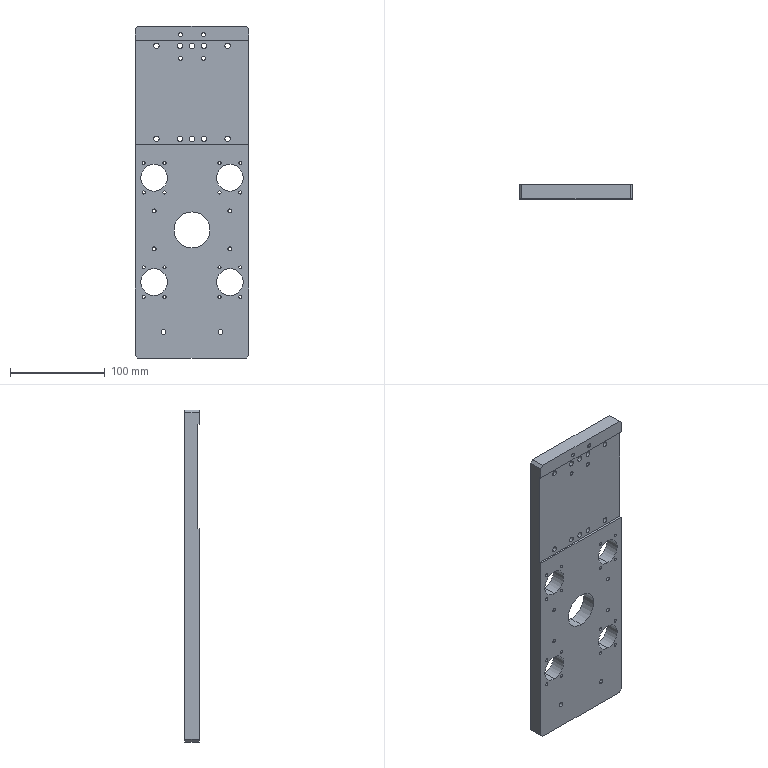Part | SolidWorks | features HoleWzd 6, Cut 2, Chamfer 1, Extrusion 1, ICE 1 | 1 solid | 120 faces | box 120 x 15 x 350 mm | volume 538843 mm3 | cylinder 98 | plane 22 | commonest cylinder face diameters 3.3 x32 4.2 x16 5.5 x16 10 x16 28.2 x8 5 x4